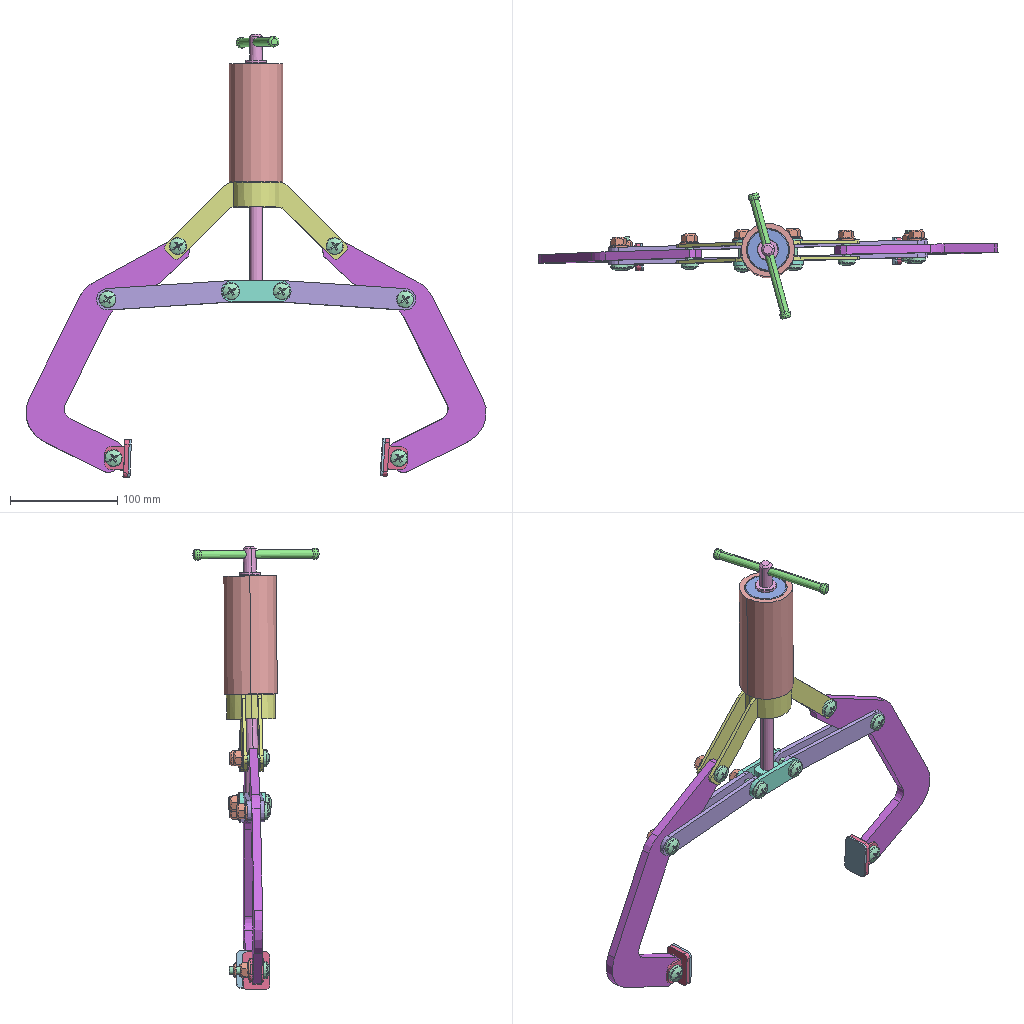Assembly | SolidWorks | 14 different items | 20 placed | box 429 x 118 x 413 mm
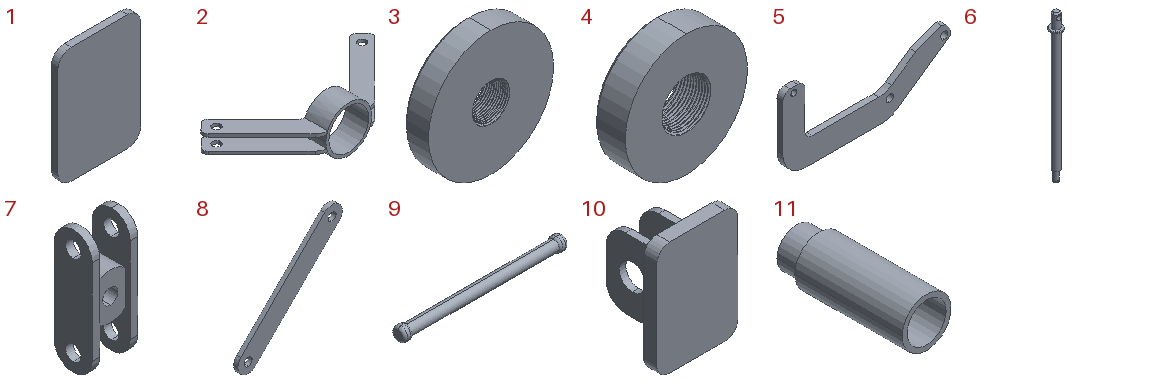Parts list (item | name | quantity | size | volume | features):
1 | - | x2 | 25 x 2 x 35 mm | 1723 mm3 | features Extrusion 1
2 | - | x1 | 170.316 x 71.647 x 46.1 mm | 26521 mm3 | features ICE 3, CosmeticWeldCutList 1, Extrusion 1
3 | - | x1 | 39.9 x 8.112 x 39.9 mm | 9095 mm3 | features Chamfer 1, Extrusion 1, SweepThread 1
4 | - | x1 | 29.9 x 8.112 x 29.9 mm | 4725 mm3 | features Chamfer 1, Extrusion 1, SweepThread 1
5 | - | x2 | 227.652 x 7.9 x 102.468 mm | 70886 mm3 | features Extrusion 1, Fillet 1, ICE 1
6 | - | x1 | 20 x 20 x 250 mm | 27080 mm3 | features Chamfer 3, ICE 2, Revolution 1
7 | - | x1 | 24 x 20 x 65 mm | 13444 mm3 | features ICE 2, Chamfer 1, Extrusion 1, MirrorPattern 1
8 | - | x4 | 101.635 x 4 x 101.635 mm | 10090 mm3 | features Extrusion 1
9 | - | x1 | 120 x 10 x 10 mm | 6156 mm3 | features Fillet 1, ICE 1, MirrorPattern 1, Revolution 1
10 | - | x2 | 25 x 22 x 35 mm | 4732 mm3 | features ICE 2, CosmeticWeldCutList 1, Extrusion 1, Fillet 1
11 | - | x1 | 50 x 133.28 x 50 mm | 92984 mm3 | features Revolution 1
12 | e-ring external retaining ring_am | x1 | - | - | -
13 | pan cross head_am | x1 | - | - | -
14 | prevailing torque hex flange nut_am | x1 | - | - | -
Mates (type | each side: item.copy, entity, surface, feature):
Concentric | 11.1 face cylinder Revolve1 | 4.1 face cylinder Boss.-Extru.1
Coincident | 11.1 face plane Revolve1 | 4.1 face plane Boss.-Extru.1
Concentric | 11.1 face cylinder Revolve1 | 3.1 face cylinder Boss.-Extru.1
Concentric | 11.1 face cylinder Revolve1 | 6.1 face cylinder Revolve1
Concentric | 6.1 face cylinder Revolve1 | 7.1 face cylinder Boss.-Extru.1
Coincident | 6.1 face plane Revolve1 | 7.1 face plane Boss.-Extru.1
Concentric | 7.1 face cylinder Mirror1 | 8.1 face cylinder Boss.-Extru.1
Concentric | 7.1 face cylinder Mirror1 | 8.2 face cylinder Boss.-Extru.1
Concentric | 7.1 face cylinder Mirror1 | 8.3 face cylinder Boss.-Extru.1
Concentric | 7.1 face cylinder Mirror1 | 8.4 face cylinder Boss.-Extru.1
Coincident | 7.1 face plane Mirror1 | 8.4 face plane Boss.-Extru.1
Coincident | 7.1 face plane Boss.-Extru.4 | 8.2 face plane Boss.-Extru.1
Coincident | 7.1 face plane Mirror1 | 8.3 face plane Boss.-Extru.1
Coincident | 7.1 face plane Boss.-Extru.4 | 8.1 face plane Boss.-Extru.1
Coincident | 10.1 face plane Boss.-Extru.1 | 1.1 face plane Boss.-Extru.1 | 3 times
Coincident | 10.2 face plane Boss.-Extru.1 | 1.2 face plane Boss.-Extru.1 | 3 times
Concentric | 11.1 face cylinder Revolve1 | 2.1 face cylinder Cut-Extrude1
Coincident | 11.1 face plane Revolve1 | 2.1 face plane Boss.-Extru.2
Concentric | 2.1 face cylinder Boss.-Extru.1 | 5.1 face cylinder Boss.-Extru.1
Concentric | 8.1 face cylinder Boss.-Extru.1 | 5.1 face cylinder Cut-Extrude1
Concentric | 8.3 face cylinder Boss.-Extru.1 | 5.1 face cylinder Cut-Extrude1
Coincident | 8.1 face plane Boss.-Extru.1 | 5.1 face plane Boss.-Extru.1
Concentric | 10.1 face cylinder Cut-Extrude1 | 5.1 face cylinder Boss.-Extru.1
Concentric | 2.1 face cylinder Boss.-Extru.1 | 5.2 face cylinder Boss.-Extru.1
Concentric | 8.2 face cylinder Boss.-Extru.1 | 5.2 face cylinder Cut-Extrude1
Concentric | 8.4 face cylinder Boss.-Extru.1 | 5.2 face cylinder Cut-Extrude1
Coincident | 8.2 face plane Boss.-Extru.1 | 5.2 face plane Boss.-Extru.1
Concentric | 10.2 face cylinder Cut-Extrude1 | 5.2 face cylinder Boss.-Extru.1
Coincident | 10.2 face plane Boss.-Extru.2 | 5.2 face plane Boss.-Extru.1
Coincident | 10.1 face plane Boss.-Extru.2 | 5.1 face plane Boss.-Extru.1
Coincident | 11.1 face plane Revolve1 | 3.1 face plane Boss.-Extru.1
Concentric | 6.1 face cylinder Cut-Extrude2 | 9.1 face cylinder Revolve1